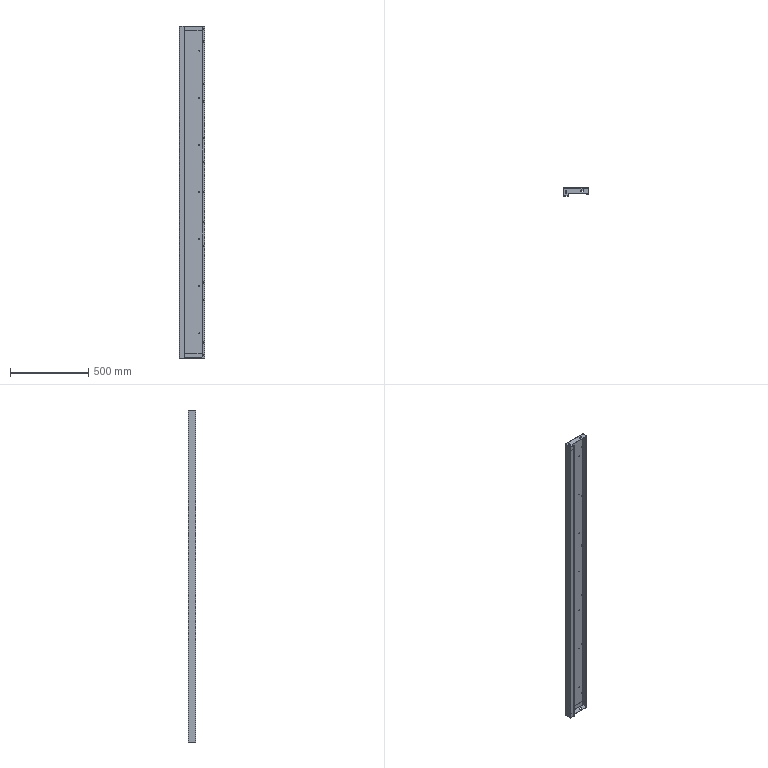Part | SolidWorks | features MirrorCompFeat 1, ReferencePattern 1 | 3 solids | 212 faces | box 160.5 x 50 x 2116 mm | volume 792691 mm3 | plane 114 | cylinder 98 | commonest cylinder face diameters 6.2 x28 4.2 x14 8 x12 11 x12 1 x11 10 x10